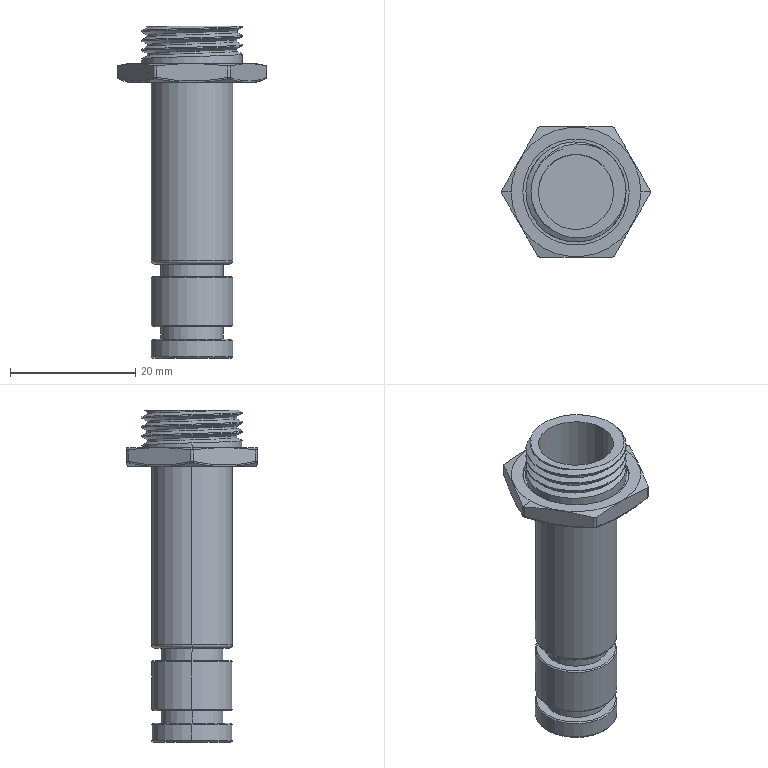Part | SolidWorks | features Cut 4, Fillet 4, ICE 2, Chamfer 1, Extrusion 1, RefAxis 1, RevCut 1, SweepThread 1 | 1 solid | 81 faces | box 23.845 x 20.785 x 53 mm | volume 4184 mm3 | cylinder 30 | plane 17 | cone 15 | spline 15 | torus 4 | commonest cylinder face diameters 16 x9 1 x7 13 x6 10 x4 12 x2 17 x2